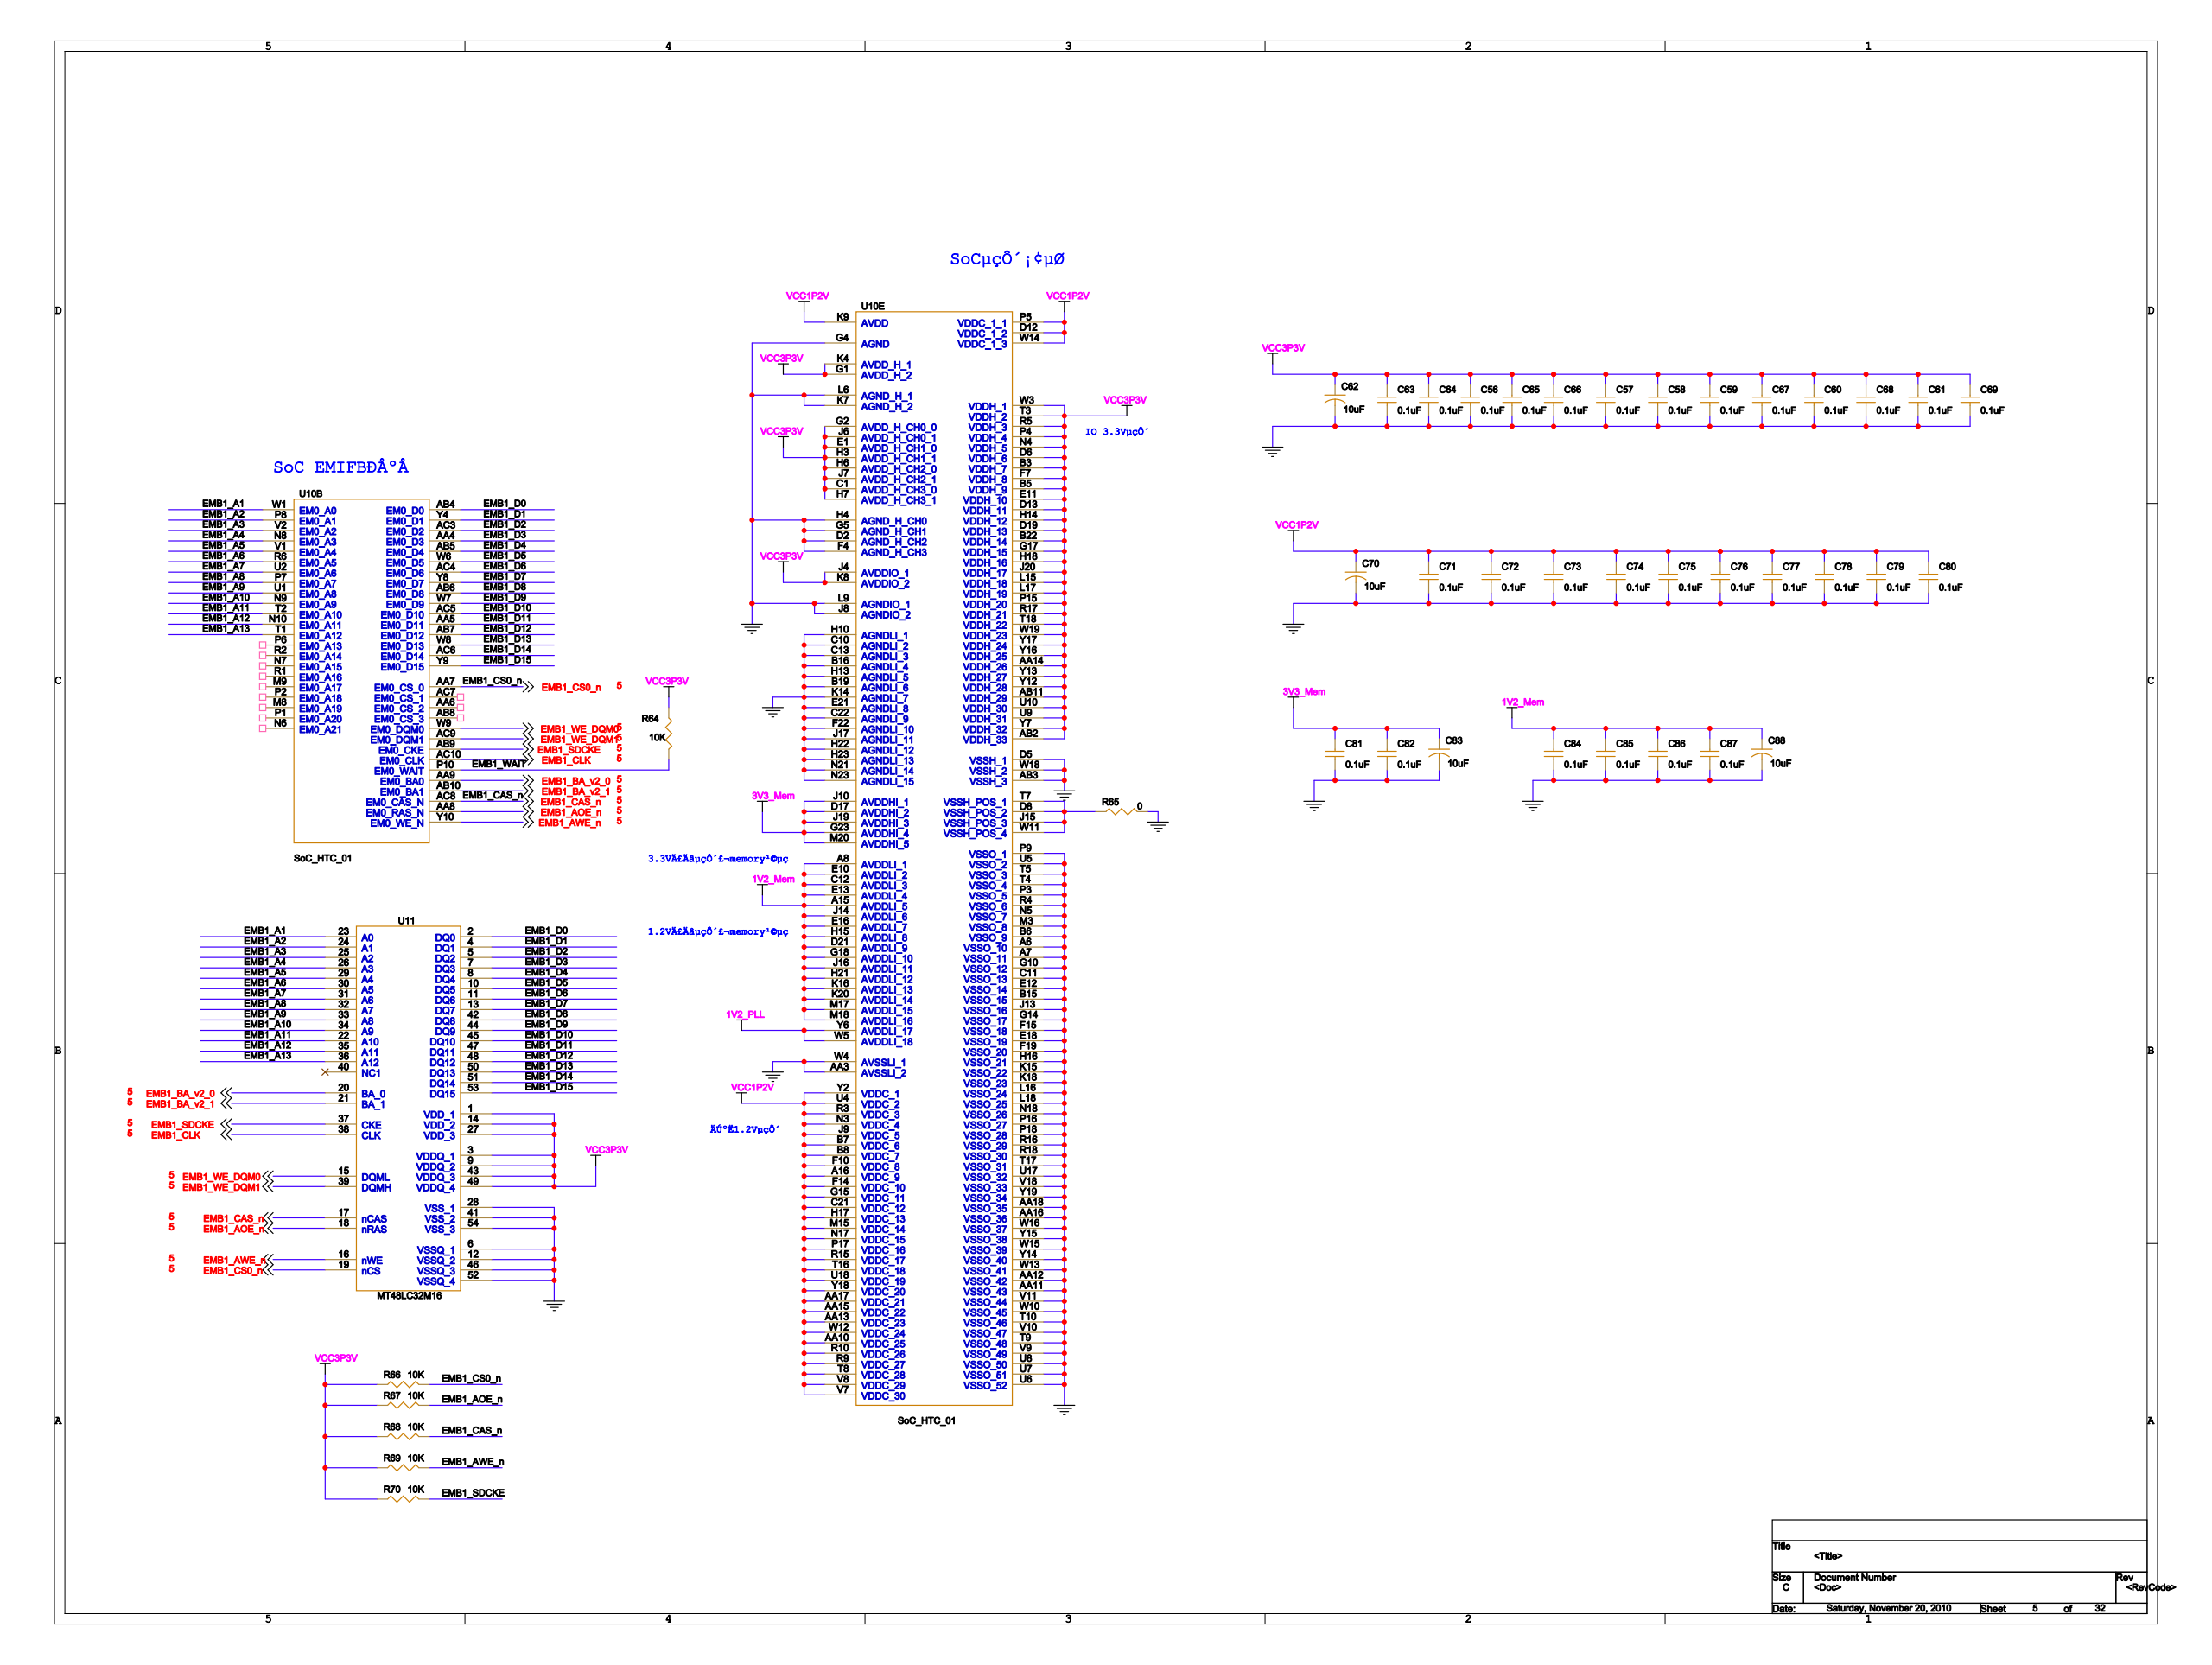Circuit board | Cadence Allegro | 1001 parts | 1318 nets | one sheet of the schematic
Parts on this sheet (reference | value | footprint):
C56 | 0.1uF | C0402
C57 | 0.1uF | C0402
C58 | 0.1uF | C0402
C59 | 0.1uF | C0402
C60 | 0.1uF | C0402
C61 | 0.1uF | C0402
C62 | 10uF | C3216
C63 | 0.1uF | C0402
C64 | 0.1uF | C0402
C65 | 0.1uF | C0402
C66 | 0.1uF | C0402
C67 | 0.1uF | C0402
C68 | 0.1uF | C0402
C69 | 0.1uF | C0402
C70 | 10uF | C3216
C71 | 0.1uF | C0402
C72 | 0.1uF | C0402
C73 | 0.1uF | C0402
C74 | 0.1uF | C0402
C75 | 0.1uF | C0402
C76 | 0.1uF | C0402
C77 | 0.1uF | C0402
C78 | 0.1uF | C0402
C79 | 0.1uF | C0402
C80 | 0.1uF | C0402
C81 | 0.1uF | C0402
C82 | 0.1uF | C0402
C83 | 10uF | C3216
C84 | 0.1uF | C0402
C85 | 0.1uF | C0402
C86 | 0.1uF | C0402
C87 | 0.1uF | C0402
C88 | 10uF | C3216
R64 | 10K | 0603
R65 | 0 | 0603
R66 | 10K | 0603
R67 | 10K | 0603
R68 | 10K | 0603
R69 | 10K | 0603
R70 | 10K | 0603
U1 | SoC_HTC_01 | L529_XIN
U2 | MT48LC32M16 | TSOP54
U4 | MAX3243 | TSSOP-28
U6 | MT48LC16M16 | TSOP54
U7 | MT48LC16M16 | TSOP54
U8 | DP83848C | DP83848C_48LQFP
U10 | SoC_HTC_01 | L529_XIN
U11 | MT48LC32M16 | TSOP54
U17 | MT48LC32M16 | TSOP54
Nets of these parts (net: part-pin ...):
GND: C56-2 C57-2 C58-2 C59-2 C60-2 C61-2 C62-2 C63-2 C64-2 C65-2 C66-2 C67-2 C68-2 C69-2 C70-2 C71-2 C72-2 C73-2 C74-2 C75-2 C76-2 C77-2 C78-2 C79-2 C80-2 C81-2 C82-2 C83-2 C84-2 C85-2 C86-2 C87-2 C88-2 R65-2 U1-A6 U1-A7 U1-AA3 U1-AA11 U1-AA12 U1-AA16 U1-AA18 U1-AB3 U1-B6 U1-B15 U1-B16 U1-B19 U1-C10 U1-C11 U1-C13 U1-C22 U1-D2 U1-D5 U1-E12 U1-E18 U1-E21 U1-F4 U1-F15 U1-F19 U1-F22 U1-G4 U1-G5 U1-G10 U1-G14 U1-H4 U1-H10 U1-H13 U1-H16 U1-H22 U1-H23 U1-J8 U1-J13 U1-J17 U1-K7 U1-K14 U1-K15 U1-K18 U1-L6 U1-L9 U1-L16 U1-L18 U1-M3 U1-N5 U1-N18 U1-N21 U1-N23 U1-P3 U1-P9 U1-P16 U1-P18 U1-R4 U1-R16 U1-R18 U1-T4 U1-T5 U1-T9 U1-T10 U1-T17 U1-U5 U1-U6 U1-U7 U1-U8 U1-U17 U1-V9 U1-V10 U1-V11 U1-V18 U1-W4 U1-W10 U1-W13 U1-W15 U1-W16 U1-W18 U1-Y14 U1-Y15 U1-Y19 U2-6 U2-12 U2-28 U2-41 U2-46 U2-52 U2-54 U4-23 U4-25 U6-6 U6-12 U6-28 U6-41 U6-46 U6-52 U6-54 U7-6 U7-12 U7-28 U7-41 U7-46 U7-52 U7-54 U8-15 U8-19 U8-35 U8-36 U8-47 U10-A6 U10-A7 U10-AA3 U10-AA11 U10-AA12 U10-AA16 U10-AA18 U10-AB3 U10-B6 U10-B15 U10-B16 U10-B19 U10-C10 U10-C11 U10-C13 U10-C22 U10-D2 U10-D5 U10-E12 U10-E18 U10-E21 U10-F4 U10-F15 U10-F19 U10-F22 U10-G4 U10-G5 U10-G10 U10-G14 U10-H4 U10-H10 U10-H13 U10-H16 U10-H22 U10-H23 U10-J8 U10-J13 U10-J17 U10-K7 U10-K14 U10-K15 U10-K18 U10-L6 U10-L9 U10-L16 U10-L18 U10-M3 U10-N5 U10-N18 U10-N21 U10-N23 U10-P3 U10-P9 U10-P16 U10-P18 U10-R4 U10-R16 U10-R18 U10-T4 U10-T5 U10-T9 U10-T10 U10-T17 U10-U5 U10-U6 U10-U7 U10-U8 U10-U17 U10-V9 U10-V10 U10-V11 U10-V18 U10-W4 U10-W10 U10-W13 U10-W15 U10-W16 U10-W18 U10-Y14 U10-Y15 U10-Y19 U11-6 U11-12 U11-28 U11-41 U11-46 U11-52 U11-54 U17-6 U17-12 U17-28 U17-41 U17-46 U17-52 U17-54
VCC3P3V: C56-1 C57-1 C58-1 C59-1 C60-1 C61-1 C62-1 C63-1 C64-1 C65-1 C66-1 C67-1 C68-1 C69-1 R64-2 R66-1 R67-1 R68-1 R69-1 R70-1 U1-AA14 U1-AB2 U1-AB11 U1-B3 U1-B5 U1-B22 U1-C1 U1-D6 U1-D13 U1-D19 U1-E1 U1-E11 U1-F7 U1-G1 U1-G2 U1-G17 U1-H3 U1-H6 U1-H7 U1-H14 U1-H18 U1-J4 U1-J6 U1-J7 U1-J20 U1-K4 U1-K8 U1-L15 U1-L17 U1-N4 U1-P4 U1-P15 U1-R5 U1-R17 U1-T3 U1-T18 U1-U9 U1-U10 U1-W3 U1-W19 U1-Y7 U1-Y12 U1-Y13 U1-Y16 U1-Y17 U2-1 U2-3 U2-9 U2-14 U2-27 U2-43 U2-49 U4-22 U4-26 U6-1 U6-3 U6-9 U6-14 U6-27 U6-43 U6-49 U7-1 U7-3 U7-9 U7-14 U7-27 U7-43 U7-49 U8-22 U8-32 U8-48 U10-AA14 U10-AB2 U10-AB11 U10-B3 U10-B5 U10-B22 U10-C1 U10-D6 U10-D13 U10-D19 U10-E1 U10-E11 U10-F7 U10-G1 U10-G2 U10-G17 U10-H3 U10-H6 U10-H7 U10-H14 U10-H18 U10-J4 U10-J6 U10-J7 U10-J20 U10-K4 U10-K8 U10-L15 U10-L17 U10-N4 U10-P4 U10-P15 U10-R5 U10-R17 U10-T3 U10-T18 U10-U9 U10-U10 U10-W3 U10-W19 U10-Y7 U10-Y12 U10-Y13 U10-Y16 U10-Y17 U11-1 U11-3 U11-9 U11-14 U11-27 U11-43 U11-49 U17-1 U17-3 U17-9 U17-14 U17-27 U17-43 U17-49
VCC1P2V: C70-1 C71-1 C72-1 C73-1 C74-1 C75-1 C76-1 C77-1 C78-1 C79-1 C80-1 U1-A16 U1-AA10 U1-AA13 U1-AA15 U1-AA17 U1-B7 U1-B8 U1-C21 U1-D12 U1-F10 U1-F14 U1-G15 U1-H17 U1-J9 U1-K9 U1-M15 U1-N3 U1-N17 U1-P5 U1-P17 U1-R3 U1-R9 U1-R10 U1-R15 U1-T8 U1-T16 U1-U4 U1-U18 U1-V7 U1-V8 U1-W12 U1-W14 U1-Y2 U1-Y18 U10-A16 U10-AA10 U10-AA13 U10-AA15 U10-AA17 U10-B7 U10-B8 U10-C21 U10-D12 U10-F10 U10-F14 U10-G15 U10-H17 U10-J9 U10-K9 U10-M15 U10-N3 U10-N17 U10-P5 U10-P17 U10-R3 U10-R9 U10-R10 U10-R15 U10-T8 U10-T16 U10-U4 U10-U18 U10-V7 U10-V8 U10-W12 U10-W14 U10-Y2 U10-Y18
3V3_MEM: C81-1 C82-1 C83-1 U1-D17 U1-G23 U1-J10 U1-J19 U1-M20 U10-D17 U10-G23 U10-J10 U10-J19 U10-M20
1V2_MEM: C84-1 C85-1 C86-1 C87-1 C88-1 U1-A8 U1-A15 U1-C12 U1-D21 U1-E10 U1-E13 U1-E16 U1-G18 U1-H15 U1-H21 U1-J14 U1-J16 U1-K16 U1-K20 U1-M17 U1-M18 U10-A8 U10-A15 U10-C12 U10-D21 U10-E10 U10-E13 U10-E16 U10-G18 U10-H15 U10-H21 U10-J14 U10-J16 U10-K16 U10-K20 U10-M17 U10-M18
1V2_PLL: U1-W5 U1-Y6 U10-W5 U10-Y6
EMB1_A1: U10-W1 U11-23
EMB1_A2: U10-P8 U11-24
EMB1_A11: U10-T2 U11-22
EMB1_A12: U10-N10 U11-35
EMB1_A13: U10-T1 U11-36
EMB1_A3: U10-V2 U11-25
EMB1_A4: U10-N8 U11-26
EMB1_A5: U10-V1 U11-29
EMB1_A6: U10-R6 U11-30
EMB1_A7: U10-U2 U11-31
EMB1_A8: U10-P7 U11-32
EMB1_A9: U10-U1 U11-33
EMB1_A10: U10-N9 U11-34
EMB1_CAS_N: R68-2 U10-AC8 U11-17
EMB1_SDCKE: R70-2 U10-AB9 U11-37
EMB1_CLK: U10-AC10 U11-38
EMB1_CS0_N: R66-2 U10-AA7 U11-19
EMB1_D0: U10-AB4 U11-2
EMB1_D1: U10-Y4 U11-4
EMB1_D10: U10-AC5 U11-45
EMB1_D11: U10-AA5 U11-47
EMB1_D12: U10-AB7 U11-48
EMB1_D13: U10-W8 U11-50
EMB1_D14: U10-AC6 U11-51
EMB1_D15: U10-Y9 U11-53
EMB1_D2: U10-AC3 U11-5
EMB1_D3: U10-AA4 U11-7
EMB1_D4: U10-AB5 U11-8
EMB1_D5: U10-W6 U11-10
EMB1_D6: U10-AC4 U11-11
EMB1_D7: U10-Y8 U11-13
EMB1_D8: U10-AB6 U11-42
EMB1_D9: U10-W7 U11-44
EMB1_WE_DQM0: U10-W9 U11-15
EMB1_WE_DQM1: U10-AC9 U11-39
EMB1_AOE_N: R67-2 U10-AA8 U11-18
EMB1_WAIT: R64-1 U10-P10
EMB1_AWE_N: R69-2 U10-Y10 U11-16
N17396440: R65-1 U10-D8 U10-J15 U10-T7 U10-W11